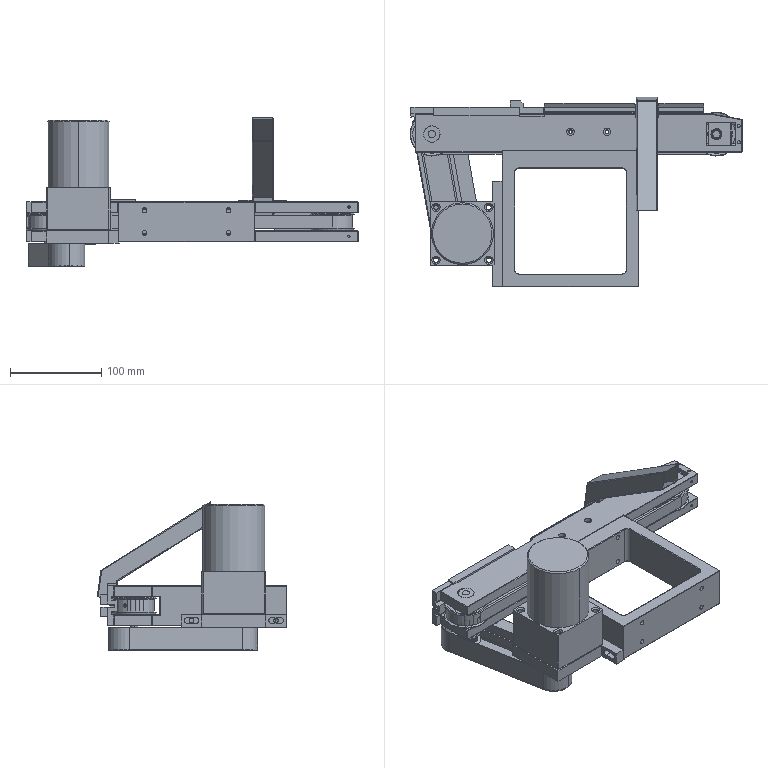Part | NX | features BREP 28 | 58 solids | 2066 faces | box 364 x 207.912 x 162.646 mm | volume 1437084 mm3 | cylinder 929 | plane 869 | cone 188 | torus 62 | sphere 18 | commonest cylinder face diameters 1.22 x152 1.06 x69 1.72 x68 5 x62 3.3 x56 8 x50